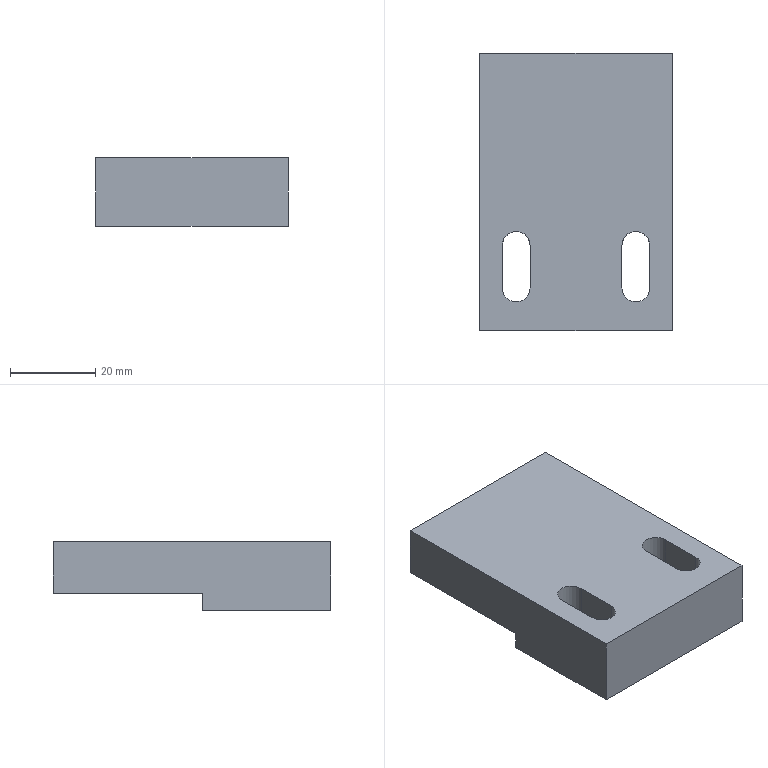Part | STEP file | top shaft cylinder seat support plate 2 | 1 solid | 24 faces | box 45 x 65 x 16 mm | volume 36671 mm3 | plane 12 | cylinder 8 | cone 4 | commonest cylinder face diameters 5 x4 6.5 x4